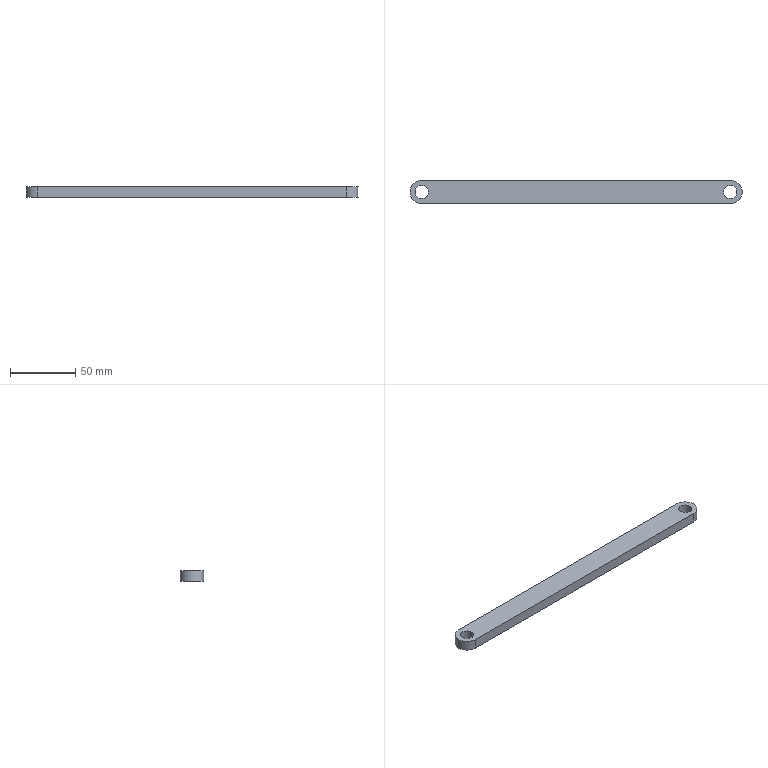Part | STEP file | Connecting rod | 1 solid | 8 faces | box 254.04 x 18 x 8 mm | volume 34769 mm3 | plane 4 | cylinder 4 | commonest cylinder face diameters 10 x2 18 x2
STEP:
#1=CARTESIAN_POINT('',(0.,0.,0.));
#2=DIRECTION('',(0.,0.,1.));
#3=DIRECTION('',(1.,0.,0.));
#4=AXIS2_PLACEMENT_3D('',#1,#2,#3);
#5=CARTESIAN_POINT('',(241.04,0.,8.));
#6=VERTEX_POINT('',#5);
#7=CARTESIAN_POINT('',(236.04,0.,8.));
#8=DIRECTION('',(0.,0.,1.));
#9=DIRECTION('',(1.,0.,0.));
#10=AXIS2_PLACEMENT_3D('',#7,#8,#9);
#11=CIRCLE('',#10,5.);
#12=CARTESIAN_POINT('',(0.,0.,8.));
#13=DIRECTION('',(0.,0.,1.));
#14=DIRECTION('',(1.,0.,0.));
#15=AXIS2_PLACEMENT_3D('',#12,#13,#14);
#16=PLANE('',#15);
#17=CARTESIAN_POINT('',(236.04,0.));
#18=DIRECTION('',(1.,0.));
#19=AXIS2_PLACEMENT_2D('',#17,#18);
#20=CIRCLE('',#19,5.);
#21=(GEOMETRIC_REPRESENTATION_CONTEXT(2)PARAMETRIC_REPRESENTATION_CONTEXT()REPRESENTATION_CONTEXT('',''));
#22=DEFINITIONAL_REPRESENTATION('',(#20),#21);
#23=PCURVE('',#16,#22);
#24=CARTESIAN_POINT('',(236.04,0.,8.));
#25=DIRECTION('',(0.,0.,-1.));
#26=DIRECTION('',(-1.,0.,0.));
#27=AXIS2_PLACEMENT_3D('',#24,#25,#26);
#28=CYLINDRICAL_SURFACE('',#27,5.);
#29=CARTESIAN_POINT('',(9.425,0.));
#30=DIRECTION('',(-1.,0.));
#31=VECTOR('',#30,1.);
#32=LINE('',#29,#31);
#33=(GEOMETRIC_REPRESENTATION_CONTEXT(2)PARAMETRIC_REPRESENTATION_CONTEXT()REPRESENTATION_CONTEXT('',''));
#34=DEFINITIONAL_REPRESENTATION('',(#32),#33);
#35=PCURVE('',#28,#34);
#36=SURFACE_CURVE('',#11,(#23,#35),.PCURVE_S1.);
#37=EDGE_CURVE('',#6,#6,#36,.T.);
#38=ORIENTED_EDGE('',*,*,#37,.F.);
#39=EDGE_LOOP('',(#38));
#40=FACE_BOUND('',#39,.T.);
#41=CARTESIAN_POINT('',(0.,9.,8.));
#42=VERTEX_POINT('',#41);
#43=CARTESIAN_POINT('',(0.,-9.,8.));
#44=VERTEX_POINT('',#43);
#45=CARTESIAN_POINT('',(0.,0.,8.));
#46=DIRECTION('',(0.,0.,1.));
#47=DIRECTION('',(1.,0.,0.));
#48=AXIS2_PLACEMENT_3D('',#45,#46,#47);
#49=CIRCLE('',#48,9.);
#50=CARTESIAN_POINT('',(0.,0.));
#51=DIRECTION('',(1.,0.));
#52=AXIS2_PLACEMENT_2D('',#50,#51);
#53=CIRCLE('',#52,9.);
#54=(GEOMETRIC_REPRESENTATION_CONTEXT(2)PARAMETRIC_REPRESENTATION_CONTEXT()REPRESENTATION_CONTEXT('',''));
#55=DEFINITIONAL_REPRESENTATION('',(#53),#54);
#56=PCURVE('',#16,#55);
#57=CARTESIAN_POINT('',(0.,0.,8.));
#58=DIRECTION('',(0.,0.,-1.));
#59=DIRECTION('',(-1.,0.,0.));
#60=AXIS2_PLACEMENT_3D('',#57,#58,#59);
#61=CYLINDRICAL_SURFACE('',#60,9.);
#62=CARTESIAN_POINT('',(3.142,0.));
#63=DIRECTION('',(-1.,0.));
#64=VECTOR('',#63,1.);
#65=LINE('',#62,#64);
#66=(GEOMETRIC_REPRESENTATION_CONTEXT(2)PARAMETRIC_REPRESENTATION_CONTEXT()REPRESENTATION_CONTEXT('',''));
#67=DEFINITIONAL_REPRESENTATION('',(#65),#66);
#68=PCURVE('',#61,#67);
#69=SURFACE_CURVE('',#49,(#56,#68),.PCURVE_S1.);
#70=EDGE_CURVE('',#42,#44,#69,.T.);
#71=ORIENTED_EDGE('',*,*,#70,.T.);
#72=CARTESIAN_POINT('',(236.04,-9.,8.));
#73=VERTEX_POINT('',#72);
#74=CARTESIAN_POINT('',(0.,-9.,8.));
#75=DIRECTION('',(1.,0.,0.));
#76=VECTOR('',#75,1.);
#77=LINE('',#74,#76);
#78=CARTESIAN_POINT('',(0.,-9.));
#79=DIRECTION('',(1.,0.));
#80=VECTOR('',#79,1.);
#81=LINE('',#78,#80);
#82=(GEOMETRIC_REPRESENTATION_CONTEXT(2)PARAMETRIC_REPRESENTATION_CONTEXT()REPRESENTATION_CONTEXT('',''));
#83=DEFINITIONAL_REPRESENTATION('',(#81),#82);
#84=PCURVE('',#16,#83);
#85=CARTESIAN_POINT('',(0.,-9.,8.));
#86=DIRECTION('',(0.,1.,0.));
#87=DIRECTION('',(0.,0.,1.));
#88=AXIS2_PLACEMENT_3D('',#85,#86,#87);
#89=PLANE('',#88);
#90=CARTESIAN_POINT('',(0.,0.));
#91=DIRECTION('',(0.,1.));
#92=VECTOR('',#91,1.);
#93=LINE('',#90,#92);
#94=(GEOMETRIC_REPRESENTATION_CONTEXT(2)PARAMETRIC_REPRESENTATION_CONTEXT()REPRESENTATION_CONTEXT('',''));
#95=DEFINITIONAL_REPRESENTATION('',(#93),#94);
#96=PCURVE('',#89,#95);
#97=SURFACE_CURVE('',#77,(#84,#96),.PCURVE_S1.);
#98=EDGE_CURVE('',#44,#73,#97,.T.);
#99=ORIENTED_EDGE('',*,*,#98,.T.);
#100=CARTESIAN_POINT('',(236.04,9.,8.));
#101=VERTEX_POINT('',#100);
#102=CARTESIAN_POINT('',(236.04,0.,8.));
#103=DIRECTION('',(0.,0.,1.));
#104=DIRECTION('',(1.,0.,0.));
#105=AXIS2_PLACEMENT_3D('',#102,#103,#104);
#106=CIRCLE('',#105,9.);
#107=CARTESIAN_POINT('',(236.04,0.));
#108=DIRECTION('',(1.,0.));
#109=AXIS2_PLACEMENT_2D('',#107,#108);
#110=CIRCLE('',#109,9.);
#111=(GEOMETRIC_REPRESENTATION_CONTEXT(2)PARAMETRIC_REPRESENTATION_CONTEXT()REPRESENTATION_CONTEXT('',''));
#112=DEFINITIONAL_REPRESENTATION('',(#110),#111);
#113=PCURVE('',#16,#112);
#114=CARTESIAN_POINT('',(236.04,0.,8.));
#115=DIRECTION('',(0.,0.,-1.));
#116=DIRECTION('',(-1.,0.,0.));
#117=AXIS2_PLACEMENT_3D('',#114,#115,#116);
#118=CYLINDRICAL_SURFACE('',#117,9.);
#119=CARTESIAN_POINT('',(9.425,0.));
#120=DIRECTION('',(-1.,0.));
#121=VECTOR('',#120,1.);
#122=LINE('',#119,#121);
#123=(GEOMETRIC_REPRESENTATION_CONTEXT(2)PARAMETRIC_REPRESENTATION_CONTEXT()REPRESENTATION_CONTEXT('',''));
#124=DEFINITIONAL_REPRESENTATION('',(#122),#123);
#125=PCURVE('',#118,#124);
#126=SURFACE_CURVE('',#106,(#113,#125),.PCURVE_S1.);
#127=EDGE_CURVE('',#73,#101,#126,.T.);
#128=ORIENTED_EDGE('',*,*,#127,.T.);
#129=CARTESIAN_POINT('',(0.,9.,8.));
#130=DIRECTION('',(-1.,0.,0.));
#131=VECTOR('',#130,1.);
#132=LINE('',#129,#131);
#133=CARTESIAN_POINT('',(0.,9.));
#134=DIRECTION('',(-1.,0.));
#135=VECTOR('',#134,1.);
#136=LINE('',#133,#135);
#137=(GEOMETRIC_REPRESENTATION_CONTEXT(2)PARAMETRIC_REPRESENTATION_CONTEXT()REPRESENTATION_CONTEXT('',''));
#138=DEFINITIONAL_REPRESENTATION('',(#136),#137);
#139=PCURVE('',#16,#138);
#140=CARTESIAN_POINT('',(0.,9.,8.));
#141=DIRECTION('',(0.,-1.,0.));
#142=DIRECTION('',(0.,0.,-1.));
#143=AXIS2_PLACEMENT_3D('',#140,#141,#142);
#144=PLANE('',#143);
#145=CARTESIAN_POINT('',(0.,0.));
#146=DIRECTION('',(0.,-1.));
#147=VECTOR('',#146,1.);
#148=LINE('',#145,#147);
#149=(GEOMETRIC_REPRESENTATION_CONTEXT(2)PARAMETRIC_REPRESENTATION_CONTEXT()REPRESENTATION_CONTEXT('',''));
#150=DEFINITIONAL_REPRESENTATION('',(#148),#149);
#151=PCURVE('',#144,#150);
#152=SURFACE_CURVE('',#132,(#139,#151),.PCURVE_S1.);
#153=EDGE_CURVE('',#101,#42,#152,.T.);
#154=ORIENTED_EDGE('',*,*,#153,.T.);
#155=EDGE_LOOP('',(#71,#99,#128,#154));
#156=FACE_BOUND('',#155,.T.);
#157=CARTESIAN_POINT('',(5.,0.,8.));
#158=VERTEX_POINT('',#157);
#159=CARTESIAN_POINT('',(0.,0.,8.));
#160=DIRECTION('',(0.,0.,1.));
#161=DIRECTION('',(1.,0.,0.));
#162=AXIS2_PLACEMENT_3D('',#159,#160,#161);
#163=CIRCLE('',#162,5.);
#164=CARTESIAN_POINT('',(0.,0.));
#165=DIRECTION('',(1.,0.));
#166=AXIS2_PLACEMENT_2D('',#164,#165);
#167=CIRCLE('',#166,5.);
#168=(GEOMETRIC_REPRESENTATION_CONTEXT(2)PARAMETRIC_REPRESENTATION_CONTEXT()REPRESENTATION_CONTEXT('',''));
#169=DEFINITIONAL_REPRESENTATION('',(#167),#168);
#170=PCURVE('',#16,#169);
#171=CARTESIAN_POINT('',(0.,0.,8.));
#172=DIRECTION('',(0.,0.,-1.));
#173=DIRECTION('',(-1.,0.,0.));
#174=AXIS2_PLACEMENT_3D('',#171,#172,#173);
#175=CYLINDRICAL_SURFACE('',#174,5.);
#176=CARTESIAN_POINT('',(9.425,0.));
#177=DIRECTION('',(-1.,0.));
#178=VECTOR('',#177,1.);
#179=LINE('',#176,#178);
#180=(GEOMETRIC_REPRESENTATION_CONTEXT(2)PARAMETRIC_REPRESENTATION_CONTEXT()REPRESENTATION_CONTEXT('',''));
#181=DEFINITIONAL_REPRESENTATION('',(#179),#180);
#182=PCURVE('',#175,#181);
#183=SURFACE_CURVE('',#163,(#170,#182),.PCURVE_S1.);
#184=EDGE_CURVE('',#158,#158,#183,.T.);
#185=ORIENTED_EDGE('',*,*,#184,.F.);
#186=EDGE_LOOP('',(#185));
#187=FACE_BOUND('',#186,.T.);
#188=ADVANCED_FACE('',(#40,#156,#187),#16,.T.);
#189=CARTESIAN_POINT('',(0.,9.,0.));
#190=VERTEX_POINT('',#189);
#191=CARTESIAN_POINT('',(0.,-9.,0.));
#192=VERTEX_POINT('',#191);
#193=CARTESIAN_POINT('',(0.,0.,0.));
#194=DIRECTION('',(0.,0.,1.));
#195=DIRECTION('',(1.,0.,0.));
#196=AXIS2_PLACEMENT_3D('',#193,#194,#195);
#197=CIRCLE('',#196,9.);
#198=CARTESIAN_POINT('',(0.,0.,0.));
#199=DIRECTION('',(0.,0.,1.));
#200=DIRECTION('',(1.,0.,0.));
#201=AXIS2_PLACEMENT_3D('',#198,#199,#200);
#202=PLANE('',#201);
#203=CARTESIAN_POINT('',(0.,0.));
#204=DIRECTION('',(1.,0.));
#205=AXIS2_PLACEMENT_2D('',#203,#204);
#206=CIRCLE('',#205,9.);
#207=(GEOMETRIC_REPRESENTATION_CONTEXT(2)PARAMETRIC_REPRESENTATION_CONTEXT()REPRESENTATION_CONTEXT('',''));
#208=DEFINITIONAL_REPRESENTATION('',(#206),#207);
#209=PCURVE('',#202,#208);
#210=CARTESIAN_POINT('',(3.142,8.));
#211=DIRECTION('',(-1.,0.));
#212=VECTOR('',#211,1.);
#213=LINE('',#210,#212);
#214=(GEOMETRIC_REPRESENTATION_CONTEXT(2)PARAMETRIC_REPRESENTATION_CONTEXT()REPRESENTATION_CONTEXT('',''));
#215=DEFINITIONAL_REPRESENTATION('',(#213),#214);
#216=PCURVE('',#61,#215);
#217=SURFACE_CURVE('',#197,(#209,#216),.PCURVE_S1.);
#218=EDGE_CURVE('',#190,#192,#217,.T.);
#219=ORIENTED_EDGE('',*,*,#218,.F.);
#220=CARTESIAN_POINT('',(236.04,9.,0.));
#221=VERTEX_POINT('',#220);
#222=CARTESIAN_POINT('',(0.,9.,0.));
#223=DIRECTION('',(-1.,0.,0.));
#224=VECTOR('',#223,1.);
#225=LINE('',#222,#224);
#226=CARTESIAN_POINT('',(0.,9.));
#227=DIRECTION('',(-1.,0.));
#228=VECTOR('',#227,1.);
#229=LINE('',#226,#228);
#230=(GEOMETRIC_REPRESENTATION_CONTEXT(2)PARAMETRIC_REPRESENTATION_CONTEXT()REPRESENTATION_CONTEXT('',''));
#231=DEFINITIONAL_REPRESENTATION('',(#229),#230);
#232=PCURVE('',#202,#231);
#233=CARTESIAN_POINT('',(8.,0.));
#234=DIRECTION('',(0.,-1.));
#235=VECTOR('',#234,1.);
#236=LINE('',#233,#235);
#237=(GEOMETRIC_REPRESENTATION_CONTEXT(2)PARAMETRIC_REPRESENTATION_CONTEXT()REPRESENTATION_CONTEXT('',''));
#238=DEFINITIONAL_REPRESENTATION('',(#236),#237);
#239=PCURVE('',#144,#238);
#240=SURFACE_CURVE('',#225,(#232,#239),.PCURVE_S1.);
#241=EDGE_CURVE('',#221,#190,#240,.T.);
#242=ORIENTED_EDGE('',*,*,#241,.F.);
#243=CARTESIAN_POINT('',(236.04,-9.,0.));
#244=VERTEX_POINT('',#243);
#245=CARTESIAN_POINT('',(236.04,0.,0.));
#246=DIRECTION('',(0.,0.,1.));
#247=DIRECTION('',(1.,0.,0.));
#248=AXIS2_PLACEMENT_3D('',#245,#246,#247);
#249=CIRCLE('',#248,9.);
#250=CARTESIAN_POINT('',(236.04,0.));
#251=DIRECTION('',(1.,0.));
#252=AXIS2_PLACEMENT_2D('',#250,#251);
#253=CIRCLE('',#252,9.);
#254=(GEOMETRIC_REPRESENTATION_CONTEXT(2)PARAMETRIC_REPRESENTATION_CONTEXT()REPRESENTATION_CONTEXT('',''));
#255=DEFINITIONAL_REPRESENTATION('',(#253),#254);
#256=PCURVE('',#202,#255);
#257=CARTESIAN_POINT('',(9.425,8.));
#258=DIRECTION('',(-1.,0.));
#259=VECTOR('',#258,1.);
#260=LINE('',#257,#259);
#261=(GEOMETRIC_REPRESENTATION_CONTEXT(2)PARAMETRIC_REPRESENTATION_CONTEXT()REPRESENTATION_CONTEXT('',''));
#262=DEFINITIONAL_REPRESENTATION('',(#260),#261);
#263=PCURVE('',#118,#262);
#264=SURFACE_CURVE('',#249,(#256,#263),.PCURVE_S1.);
#265=EDGE_CURVE('',#244,#221,#264,.T.);
#266=ORIENTED_EDGE('',*,*,#265,.F.);
#267=CARTESIAN_POINT('',(0.,-9.,0.));
#268=DIRECTION('',(1.,0.,0.));
#269=VECTOR('',#268,1.);
#270=LINE('',#267,#269);
#271=CARTESIAN_POINT('',(0.,-9.));
#272=DIRECTION('',(1.,0.));
#273=VECTOR('',#272,1.);
#274=LINE('',#271,#273);
#275=(GEOMETRIC_REPRESENTATION_CONTEXT(2)PARAMETRIC_REPRESENTATION_CONTEXT()REPRESENTATION_CONTEXT('',''));
#276=DEFINITIONAL_REPRESENTATION('',(#274),#275);
#277=PCURVE('',#202,#276);
#278=CARTESIAN_POINT('',(-8.,0.));
#279=DIRECTION('',(0.,1.));
#280=VECTOR('',#279,1.);
#281=LINE('',#278,#280);
#282=(GEOMETRIC_REPRESENTATION_CONTEXT(2)PARAMETRIC_REPRESENTATION_CONTEXT()REPRESENTATION_CONTEXT('',''));
#283=DEFINITIONAL_REPRESENTATION('',(#281),#282);
#284=PCURVE('',#89,#283);
#285=SURFACE_CURVE('',#270,(#277,#284),.PCURVE_S1.);
#286=EDGE_CURVE('',#192,#244,#285,.T.);
#287=ORIENTED_EDGE('',*,*,#286,.F.);
#288=EDGE_LOOP('',(#219,#242,#266,#287));
#289=FACE_BOUND('',#288,.T.);
#290=CARTESIAN_POINT('',(241.04,0.,0.));
#291=VERTEX_POINT('',#290);
#292=CARTESIAN_POINT('',(236.04,0.,0.));
#293=DIRECTION('',(0.,0.,1.));
#294=DIRECTION('',(1.,0.,0.));
#295=AXIS2_PLACEMENT_3D('',#292,#293,#294);
#296=CIRCLE('',#295,5.);
#297=CARTESIAN_POINT('',(236.04,0.));
#298=DIRECTION('',(1.,0.));
#299=AXIS2_PLACEMENT_2D('',#297,#298);
#300=CIRCLE('',#299,5.);
#301=(GEOMETRIC_REPRESENTATION_CONTEXT(2)PARAMETRIC_REPRESENTATION_CONTEXT()REPRESENTATION_CONTEXT('',''));
#302=DEFINITIONAL_REPRESENTATION('',(#300),#301);
#303=PCURVE('',#202,#302);
#304=CARTESIAN_POINT('',(9.425,8.));
#305=DIRECTION('',(-1.,0.));
#306=VECTOR('',#305,1.);
#307=LINE('',#304,#306);
#308=(GEOMETRIC_REPRESENTATION_CONTEXT(2)PARAMETRIC_REPRESENTATION_CONTEXT()REPRESENTATION_CONTEXT('',''));
#309=DEFINITIONAL_REPRESENTATION('',(#307),#308);
#310=PCURVE('',#28,#309);
#311=SURFACE_CURVE('',#296,(#303,#310),.PCURVE_S1.);
#312=EDGE_CURVE('',#291,#291,#311,.T.);
#313=ORIENTED_EDGE('',*,*,#312,.T.);
#314=EDGE_LOOP('',(#313));
#315=FACE_BOUND('',#314,.T.);
#316=CARTESIAN_POINT('',(5.,0.,0.));
#317=VERTEX_POINT('',#316);
#318=CARTESIAN_POINT('',(0.,0.,0.));
#319=DIRECTION('',(0.,0.,1.));
#320=DIRECTION('',(1.,0.,0.));
#321=AXIS2_PLACEMENT_3D('',#318,#319,#320);
#322=CIRCLE('',#321,5.);
#323=CARTESIAN_POINT('',(0.,0.));
#324=DIRECTION('',(1.,0.));
#325=AXIS2_PLACEMENT_2D('',#323,#324);
#326=CIRCLE('',#325,5.);
#327=(GEOMETRIC_REPRESENTATION_CONTEXT(2)PARAMETRIC_REPRESENTATION_CONTEXT()REPRESENTATION_CONTEXT('',''));
#328=DEFINITIONAL_REPRESENTATION('',(#326),#327);
#329=PCURVE('',#202,#328);
#330=CARTESIAN_POINT('',(9.425,8.));
#331=DIRECTION('',(-1.,0.));
#332=VECTOR('',#331,1.);
#333=LINE('',#330,#332);
#334=(GEOMETRIC_REPRESENTATION_CONTEXT(2)PARAMETRIC_REPRESENTATION_CONTEXT()REPRESENTATION_CONTEXT('',''));
#335=DEFINITIONAL_REPRESENTATION('',(#333),#334);
#336=PCURVE('',#175,#335);
#337=SURFACE_CURVE('',#322,(#329,#336),.PCURVE_S1.);
#338=EDGE_CURVE('',#317,#317,#337,.T.);
#339=ORIENTED_EDGE('',*,*,#338,.T.);
#340=EDGE_LOOP('',(#339));
#341=FACE_BOUND('',#340,.T.);
#342=ADVANCED_FACE('',(#289,#315,#341),#202,.F.);
#343=ORIENTED_EDGE('',*,*,#218,.T.);
#344=CARTESIAN_POINT('',(0.,-9.,8.));
#345=DIRECTION('',(0.,0.,-1.));
#346=VECTOR('',#345,1.);
#347=LINE('',#344,#346);
#348=CARTESIAN_POINT('',(-1.571,0.));
#349=DIRECTION('',(0.,1.));
#350=VECTOR('',#349,1.);
#351=LINE('',#348,#350);
#352=(GEOMETRIC_REPRESENTATION_CONTEXT(2)PARAMETRIC_REPRESENTATION_CONTEXT()REPRESENTATION_CONTEXT('',''));
#353=DEFINITIONAL_REPRESENTATION('',(#351),#352);
#354=PCURVE('',#61,#353);
#355=CARTESIAN_POINT('',(0.,0.));
#356=DIRECTION('',(-1.,0.));
#357=VECTOR('',#356,1.);
#358=LINE('',#355,#357);
#359=(GEOMETRIC_REPRESENTATION_CONTEXT(2)PARAMETRIC_REPRESENTATION_CONTEXT()REPRESENTATION_CONTEXT('',''));
#360=DEFINITIONAL_REPRESENTATION('',(#358),#359);
#361=PCURVE('',#89,#360);
#362=SURFACE_CURVE('',#347,(#354,#361),.PCURVE_S1.);
#363=EDGE_CURVE('',#44,#192,#362,.T.);
#364=ORIENTED_EDGE('',*,*,#363,.F.);
#365=ORIENTED_EDGE('',*,*,#70,.F.);
#366=CARTESIAN_POINT('',(0.,9.,8.));
#367=DIRECTION('',(0.,0.,-1.));
#368=VECTOR('',#367,1.);
#369=LINE('',#366,#368);
#370=CARTESIAN_POINT('',(1.571,0.));
#371=DIRECTION('',(0.,1.));
#372=VECTOR('',#371,1.);
#373=LINE('',#370,#372);
#374=(GEOMETRIC_REPRESENTATION_CONTEXT(2)PARAMETRIC_REPRESENTATION_CONTEXT()REPRESENTATION_CONTEXT('',''));
#375=DEFINITIONAL_REPRESENTATION('',(#373),#374);
#376=PCURVE('',#61,#375);
#377=CARTESIAN_POINT('',(0.,0.));
#378=DIRECTION('',(1.,0.));
#379=VECTOR('',#378,1.);
#380=LINE('',#377,#379);
#381=(GEOMETRIC_REPRESENTATION_CONTEXT(2)PARAMETRIC_REPRESENTATION_CONTEXT()REPRESENTATION_CONTEXT('',''));
#382=DEFINITIONAL_REPRESENTATION('',(#380),#381);
#383=PCURVE('',#144,#382);
#384=SURFACE_CURVE('',#369,(#376,#383),.PCURVE_S1.);
#385=EDGE_CURVE('',#42,#190,#384,.T.);
#386=ORIENTED_EDGE('',*,*,#385,.T.);
#387=EDGE_LOOP('',(#343,#364,#365,#386));
#388=FACE_BOUND('',#387,.T.);
#389=ADVANCED_FACE('',(#388),#61,.T.);
#390=ORIENTED_EDGE('',*,*,#286,.T.);
#391=CARTESIAN_POINT('',(236.04,-9.,8.));
#392=DIRECTION('',(0.,0.,-1.));
#393=VECTOR('',#392,1.);
#394=LINE('',#391,#393);
#395=CARTESIAN_POINT('',(0.,236.04));
#396=DIRECTION('',(-1.,0.));
#397=VECTOR('',#396,1.);
#398=LINE('',#395,#397);
#399=(GEOMETRIC_REPRESENTATION_CONTEXT(2)PARAMETRIC_REPRESENTATION_CONTEXT()REPRESENTATION_CONTEXT('',''));
#400=DEFINITIONAL_REPRESENTATION('',(#398),#399);
#401=PCURVE('',#89,#400);
#402=CARTESIAN_POINT('',(4.712,0.));
#403=DIRECTION('',(0.,1.));
#404=VECTOR('',#403,1.);
#405=LINE('',#402,#404);
#406=(GEOMETRIC_REPRESENTATION_CONTEXT(2)PARAMETRIC_REPRESENTATION_CONTEXT()REPRESENTATION_CONTEXT('',''));
#407=DEFINITIONAL_REPRESENTATION('',(#405),#406);
#408=PCURVE('',#118,#407);
#409=SURFACE_CURVE('',#394,(#401,#408),.PCURVE_S1.);
#410=EDGE_CURVE('',#73,#244,#409,.T.);
#411=ORIENTED_EDGE('',*,*,#410,.F.);
#412=ORIENTED_EDGE('',*,*,#98,.F.);
#413=ORIENTED_EDGE('',*,*,#363,.T.);
#414=EDGE_LOOP('',(#390,#411,#412,#413));
#415=FACE_BOUND('',#414,.T.);
#416=ADVANCED_FACE('',(#415),#89,.F.);
#417=ORIENTED_EDGE('',*,*,#265,.T.);
#418=CARTESIAN_POINT('',(236.04,9.,8.));
#419=DIRECTION('',(0.,0.,-1.));
#420=VECTOR('',#419,1.);
#421=LINE('',#418,#420);
#422=CARTESIAN_POINT('',(1.571,0.));
#423=DIRECTION('',(0.,1.));
#424=VECTOR('',#423,1.);
#425=LINE('',#422,#424);
#426=(GEOMETRIC_REPRESENTATION_CONTEXT(2)PARAMETRIC_REPRESENTATION_CONTEXT()REPRESENTATION_CONTEXT('',''));
#427=DEFINITIONAL_REPRESENTATION('',(#425),#426);
#428=PCURVE('',#118,#427);
#429=CARTESIAN_POINT('',(0.,236.04));
#430=DIRECTION('',(1.,0.));
#431=VECTOR('',#430,1.);
#432=LINE('',#429,#431);
#433=(GEOMETRIC_REPRESENTATION_CONTEXT(2)PARAMETRIC_REPRESENTATION_CONTEXT()REPRESENTATION_CONTEXT('',''));
#434=DEFINITIONAL_REPRESENTATION('',(#432),#433);
#435=PCURVE('',#144,#434);
#436=SURFACE_CURVE('',#421,(#428,#435),.PCURVE_S1.);
#437=EDGE_CURVE('',#101,#221,#436,.T.);
#438=ORIENTED_EDGE('',*,*,#437,.F.);
#439=ORIENTED_EDGE('',*,*,#127,.F.);
#440=ORIENTED_EDGE('',*,*,#410,.T.);
#441=EDGE_LOOP('',(#417,#438,#439,#440));
#442=FACE_BOUND('',#441,.T.);
#443=ADVANCED_FACE('',(#442),#118,.T.);
#444=ORIENTED_EDGE('',*,*,#241,.T.);
#445=ORIENTED_EDGE('',*,*,#385,.F.);
#446=ORIENTED_EDGE('',*,*,#153,.F.);
#447=ORIENTED_EDGE('',*,*,#437,.T.);
#448=EDGE_LOOP('',(#444,#445,#446,#447));
#449=FACE_BOUND('',#448,.T.);
#450=ADVANCED_FACE('',(#449),#144,.F.);
#451=ORIENTED_EDGE('',*,*,#37,.F.);
#452=CARTESIAN_POINT('',(241.04,0.,8.));
#453=CARTESIAN_POINT('',(241.04,0.,0.));
#454=B_SPLINE_CURVE_WITH_KNOTS('',1,(#452,#453),.UNSPECIFIED.,.F.,.F.,(2,2),(0.,8.),.PIECEWISE_BEZIER_KNOTS.);
#455=CARTESIAN_POINT('',(9.425,0.));
#456=DIRECTION('',(0.,1.));
#457=VECTOR('',#456,1.);
#458=LINE('',#455,#457);
#459=(GEOMETRIC_REPRESENTATION_CONTEXT(2)PARAMETRIC_REPRESENTATION_CONTEXT()REPRESENTATION_CONTEXT('',''));
#460=DEFINITIONAL_REPRESENTATION('',(#458),#459);
#461=PCURVE('',#28,#460);
#462=CARTESIAN_POINT('',(3.142,0.));
#463=DIRECTION('',(0.,1.));
#464=VECTOR('',#463,1.);
#465=LINE('',#462,#464);
#466=(GEOMETRIC_REPRESENTATION_CONTEXT(2)PARAMETRIC_REPRESENTATION_CONTEXT()REPRESENTATION_CONTEXT('',''));
#467=DEFINITIONAL_REPRESENTATION('',(#465),#466);
#468=PCURVE('',#28,#467);
#469=SEAM_CURVE('',#454,(#461,#468),.PCURVE_S1.);
#470=EDGE_CURVE('',#6,#291,#469,.T.);
#471=ORIENTED_EDGE('',*,*,#470,.T.);
#472=ORIENTED_EDGE('',*,*,#312,.T.);
#473=ORIENTED_EDGE('',*,*,#470,.F.);
#474=EDGE_LOOP('',(#451,#471,#472,#473));
#475=FACE_BOUND('',#474,.F.);
#476=ADVANCED_FACE('',(#475),#28,.F.);
#477=ORIENTED_EDGE('',*,*,#184,.F.);
#478=CARTESIAN_POINT('',(5.,0.,8.));
#479=CARTESIAN_POINT('',(5.,0.,0.));
#480=B_SPLINE_CURVE_WITH_KNOTS('',1,(#478,#479),.UNSPECIFIED.,.F.,.F.,(2,2),(0.,8.),.PIECEWISE_BEZIER_KNOTS.);
#481=CARTESIAN_POINT('',(9.425,0.));
#482=DIRECTION('',(0.,1.));
#483=VECTOR('',#482,1.);
#484=LINE('',#481,#483);
#485=(GEOMETRIC_REPRESENTATION_CONTEXT(2)PARAMETRIC_REPRESENTATION_CONTEXT()REPRESENTATION_CONTEXT('',''));
#486=DEFINITIONAL_REPRESENTATION('',(#484),#485);
#487=PCURVE('',#175,#486);
#488=CARTESIAN_POINT('',(3.142,0.));
#489=DIRECTION('',(0.,1.));
#490=VECTOR('',#489,1.);
#491=LINE('',#488,#490);
#492=(GEOMETRIC_REPRESENTATION_CONTEXT(2)PARAMETRIC_REPRESENTATION_CONTEXT()REPRESENTATION_CONTEXT('',''));
#493=DEFINITIONAL_REPRESENTATION('',(#491),#492);
#494=PCURVE('',#175,#493);
#495=SEAM_CURVE('',#480,(#487,#494),.PCURVE_S1.);
#496=EDGE_CURVE('',#158,#317,#495,.T.);
#497=ORIENTED_EDGE('',*,*,#496,.T.);
#498=ORIENTED_EDGE('',*,*,#338,.T.);
#499=ORIENTED_EDGE('',*,*,#496,.F.);
#500=EDGE_LOOP('',(#477,#497,#498,#499));
#501=FACE_BOUND('',#500,.F.);
#502=ADVANCED_FACE('',(#501),#175,.F.);
#503=CLOSED_SHELL('',(#188,#342,#389,#416,#443,#450,#476,#502));
#504=MANIFOLD_SOLID_BREP('',#503);
#505=(LENGTH_UNIT()NAMED_UNIT(*)SI_UNIT(.MILLI.,.METRE.));
#506=UNCERTAINTY_MEASURE_WITH_UNIT(LENGTH_MEASURE(0.000002),#505,'','');
#507=(NAMED_UNIT(*)PLANE_ANGLE_UNIT()SI_UNIT($,.RADIAN.));
#508=(NAMED_UNIT(*)SI_UNIT($,.STERADIAN.)SOLID_ANGLE_UNIT());
#509=(GEOMETRIC_REPRESENTATION_CONTEXT(3)GLOBAL_UNCERTAINTY_ASSIGNED_CONTEXT((#506))GLOBAL_UNIT_ASSIGNED_CONTEXT((#505,#507,#508))REPRESENTATION_CONTEXT('',''));
#510=ADVANCED_BREP_SHAPE_REPRESENTATION('',(#4,#504),#509);